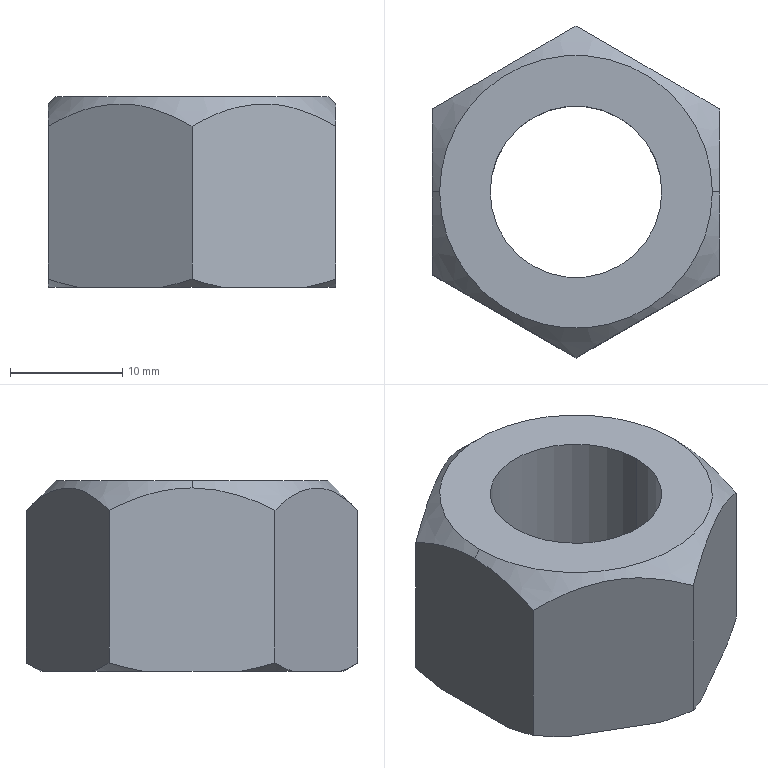Part | SolidWorks | features Cut 2, Chamfer 1, Extrusion 1 | 1 solid | 20 faces | box 25.6 x 29.56 x 17 mm | volume 6436 mm3 | cone 10 | plane 8 | cylinder 2 | commonest cylinder face diameters 15.294 x2
STEP:
#1=CARTESIAN_POINT('',(-12.15,0.,17.));
#2=VERTEX_POINT('',#1);
#3=CARTESIAN_POINT('',(12.15,0.,17.));
#4=VERTEX_POINT('',#3);
#5=CARTESIAN_POINT('',(0.,0.,17.));
#6=DIRECTION('',(0.,0.,1.));
#7=DIRECTION('',(1.,0.,0.));
#8=AXIS2_PLACEMENT_3D('',#5,#6,#7);
#9=CIRCLE('',#8,12.15);
#10=EDGE_CURVE('',#2,#4,#9,.T.);
#11=ORIENTED_EDGE('',*,*,#10,.F.);
#12=CARTESIAN_POINT('',(-12.8,0.,16.35));
#13=VERTEX_POINT('',#12);
#14=CARTESIAN_POINT('',(-12.15,0.,17.));
#15=DIRECTION('',(-0.7071,0.,-0.7071));
#16=VECTOR('',#15,1000.);
#17=LINE('',#14,#16);
#18=EDGE_CURVE('',#2,#13,#17,.T.);
#19=ORIENTED_EDGE('',*,*,#18,.T.);
#20=CARTESIAN_POINT('',(-12.8,-7.39,14.37));
#21=VERTEX_POINT('',#20);
#22=CARTESIAN_POINT('',(-12.8,0.,16.35));
#23=CARTESIAN_POINT('',(-12.8,-0.3244,16.35));
#24=CARTESIAN_POINT('',(-12.8,-0.6506,16.338));
#25=CARTESIAN_POINT('',(-12.8,-1.295,16.289));
#26=CARTESIAN_POINT('',(-12.8,-1.614,16.253));
#27=CARTESIAN_POINT('',(-12.8,-2.565,16.111));
#28=CARTESIAN_POINT('',(-12.8,-3.189,15.972));
#29=CARTESIAN_POINT('',(-12.8,-4.421,15.621));
#30=CARTESIAN_POINT('',(-12.8,-5.03,15.408));
#31=CARTESIAN_POINT('',(-12.8,-6.232,14.924));
#32=CARTESIAN_POINT('',(-12.8,-6.817,14.657));
#33=CARTESIAN_POINT('',(-12.8,-7.39,14.37));
#34=B_SPLINE_CURVE_WITH_KNOTS('',3,(#22,#23,#24,#25,#26,#27,#28,#29,#30,#31,#32,#33),.UNSPECIFIED.,.F.,.F.,(4,2,2,2,2,4),(0.01548,0.01644,0.0174,0.01931,0.02122,0.02314),.UNSPECIFIED.);
#35=EDGE_CURVE('',#13,#21,#34,.T.);
#36=ORIENTED_EDGE('',*,*,#35,.T.);
#37=CARTESIAN_POINT('',(0.,-14.78,14.37));
#38=VERTEX_POINT('',#37);
#39=CARTESIAN_POINT('',(-12.8,-7.39,14.37));
#40=CARTESIAN_POINT('',(-11.8,-7.967,14.947));
#41=CARTESIAN_POINT('',(-10.777,-8.558,15.438));
#42=CARTESIAN_POINT('',(-9.188,-9.475,15.964));
#43=CARTESIAN_POINT('',(-8.649,-9.786,16.104));
#44=CARTESIAN_POINT('',(-7.549,-10.422,16.297));
#45=CARTESIAN_POINT('',(-6.982,-10.749,16.349));
#46=CARTESIAN_POINT('',(-5.306,-11.717,16.353));
#47=CARTESIAN_POINT('',(-4.208,-12.351,16.157));
#48=CARTESIAN_POINT('',(-2.042,-13.601,15.449));
#49=CARTESIAN_POINT('',(-1.006,-14.199,14.951));
#50=CARTESIAN_POINT('',(0.,-14.78,14.37));
#51=B_SPLINE_CURVE_WITH_KNOTS('',3,(#39,#40,#41,#42,#43,#44,#45,#46,#47,#48,#49,#50),.UNSPECIFIED.,.F.,.F.,(4,2,2,2,2,4),(0.000000254,0.003817,0.005725,0.007634,0.01145,0.01527),.UNSPECIFIED.);
#52=EDGE_CURVE('',#21,#38,#51,.T.);
#53=ORIENTED_EDGE('',*,*,#52,.T.);
#54=CARTESIAN_POINT('',(12.8,-7.39,14.37));
#55=VERTEX_POINT('',#54);
#56=CARTESIAN_POINT('',(0.,-14.78,14.37));
#57=CARTESIAN_POINT('',(1.,-14.203,14.947));
#58=CARTESIAN_POINT('',(2.023,-13.612,15.438));
#59=CARTESIAN_POINT('',(3.612,-12.695,15.964));
#60=CARTESIAN_POINT('',(4.15,-12.384,16.104));
#61=CARTESIAN_POINT('',(5.251,-11.748,16.297));
#62=CARTESIAN_POINT('',(5.818,-11.421,16.349));
#63=CARTESIAN_POINT('',(7.494,-10.453,16.353));
#64=CARTESIAN_POINT('',(8.592,-9.819,16.157));
#65=CARTESIAN_POINT('',(10.758,-8.569,15.449));
#66=CARTESIAN_POINT('',(11.794,-7.971,14.951));
#67=CARTESIAN_POINT('',(12.8,-7.39,14.37));
#68=B_SPLINE_CURVE_WITH_KNOTS('',3,(#56,#57,#58,#59,#60,#61,#62,#63,#64,#65,#66,#67),.UNSPECIFIED.,.F.,.F.,(4,2,2,2,2,4),(0.000000254,0.003817,0.005725,0.007634,0.01145,0.01527),.UNSPECIFIED.);
#69=EDGE_CURVE('',#38,#55,#68,.T.);
#70=ORIENTED_EDGE('',*,*,#69,.T.);
#71=CARTESIAN_POINT('',(12.8,0.,16.35));
#72=VERTEX_POINT('',#71);
#73=CARTESIAN_POINT('',(12.8,-7.39,14.37));
#74=CARTESIAN_POINT('',(12.8,-6.817,14.657));
#75=CARTESIAN_POINT('',(12.8,-6.232,14.924));
#76=CARTESIAN_POINT('',(12.8,-5.03,15.408));
#77=CARTESIAN_POINT('',(12.8,-4.421,15.621));
#78=CARTESIAN_POINT('',(12.8,-3.189,15.972));
#79=CARTESIAN_POINT('',(12.8,-2.565,16.111));
#80=CARTESIAN_POINT('',(12.8,-1.614,16.253));
#81=CARTESIAN_POINT('',(12.8,-1.295,16.289));
#82=CARTESIAN_POINT('',(12.8,-0.6506,16.338));
#83=CARTESIAN_POINT('',(12.8,-0.3244,16.35));
#84=CARTESIAN_POINT('',(12.8,0.,16.35));
#85=B_SPLINE_CURVE_WITH_KNOTS('',3,(#73,#74,#75,#76,#77,#78,#79,#80,#81,#82,#83,#84),.UNSPECIFIED.,.F.,.F.,(4,2,2,2,2,4),(0.009846,0.01176,0.01368,0.01559,0.01655,0.0175),.UNSPECIFIED.);
#86=EDGE_CURVE('',#55,#72,#85,.T.);
#87=ORIENTED_EDGE('',*,*,#86,.T.);
#88=CARTESIAN_POINT('',(12.15,0.,17.));
#89=DIRECTION('',(0.7071,0.,-0.7071));
#90=VECTOR('',#89,1000.);
#91=LINE('',#88,#90);
#92=EDGE_CURVE('',#4,#72,#91,.T.);
#93=ORIENTED_EDGE('',*,*,#92,.F.);
#94=EDGE_LOOP('',(#11,#19,#36,#53,#70,#87,#93));
#95=FACE_OUTER_BOUND('',#94,.T.);
#96=CARTESIAN_POINT('',(0.,0.,17.));
#97=DIRECTION('',(0.,0.,-1.));
#98=DIRECTION('',(1.,0.,0.));
#99=AXIS2_PLACEMENT_3D('',#96,#97,#98);
#100=CONICAL_SURFACE('',#99,12.15,0.7854);
#101=ADVANCED_FACE('',(#95),#100,.T.);
#102=CARTESIAN_POINT('',(7.647,0.,0.2946));
#103=VERTEX_POINT('',#102);
#104=CARTESIAN_POINT('',(-7.647,0.,0.2946));
#105=VERTEX_POINT('',#104);
#106=CARTESIAN_POINT('',(0.,0.,0.2946));
#107=DIRECTION('',(0.,0.,-1.));
#108=DIRECTION('',(-1.,0.,0.));
#109=AXIS2_PLACEMENT_3D('',#106,#107,#108);
#110=CIRCLE('',#109,7.647);
#111=EDGE_CURVE('',#103,#105,#110,.T.);
#112=ORIENTED_EDGE('',*,*,#111,.F.);
#113=CARTESIAN_POINT('',(7.942,0.,0.));
#114=VERTEX_POINT('',#113);
#115=CARTESIAN_POINT('',(7.942,0.,0.));
#116=DIRECTION('',(0.7071,0.,-0.7071));
#117=VECTOR('',#116,1000.);
#118=LINE('',#115,#117);
#119=EDGE_CURVE('',#103,#114,#118,.T.);
#120=ORIENTED_EDGE('',*,*,#119,.T.);
#121=CARTESIAN_POINT('',(-7.942,0.,0.));
#122=VERTEX_POINT('',#121);
#123=CARTESIAN_POINT('',(0.,0.,0.));
#124=DIRECTION('',(0.,0.,1.));
#125=DIRECTION('',(-1.,0.,0.));
#126=AXIS2_PLACEMENT_3D('',#123,#124,#125);
#127=CIRCLE('',#126,7.942);
#128=EDGE_CURVE('',#122,#114,#127,.T.);
#129=ORIENTED_EDGE('',*,*,#128,.F.);
#130=CARTESIAN_POINT('',(-7.942,0.,0.));
#131=DIRECTION('',(-0.7071,0.,-0.7071));
#132=VECTOR('',#131,1000.);
#133=LINE('',#130,#132);
#134=EDGE_CURVE('',#105,#122,#133,.T.);
#135=ORIENTED_EDGE('',*,*,#134,.F.);
#136=EDGE_LOOP('',(#112,#120,#129,#135));
#137=FACE_OUTER_BOUND('',#136,.T.);
#138=CARTESIAN_POINT('',(0.,0.,0.));
#139=DIRECTION('',(0.,0.,-1.));
#140=DIRECTION('',(-1.,0.,0.));
#141=AXIS2_PLACEMENT_3D('',#138,#139,#140);
#142=CONICAL_SURFACE('',#141,7.942,0.7854);
#143=ADVANCED_FACE('',(#137),#142,.F.);
#144=CARTESIAN_POINT('',(-7.647,0.,17.));
#145=VERTEX_POINT('',#144);
#146=CARTESIAN_POINT('',(7.647,0.,17.));
#147=VERTEX_POINT('',#146);
#148=CARTESIAN_POINT('',(0.,0.,17.));
#149=DIRECTION('',(0.,0.,1.));
#150=DIRECTION('',(1.,0.,0.));
#151=AXIS2_PLACEMENT_3D('',#148,#149,#150);
#152=CIRCLE('',#151,7.647);
#153=EDGE_CURVE('',#145,#147,#152,.T.);
#154=ORIENTED_EDGE('',*,*,#153,.T.);
#155=CARTESIAN_POINT('',(7.647,0.,17.));
#156=DIRECTION('',(0.,0.,-1.));
#157=VECTOR('',#156,1000.);
#158=LINE('',#155,#157);
#159=EDGE_CURVE('',#147,#103,#158,.T.);
#160=ORIENTED_EDGE('',*,*,#159,.T.);
#161=ORIENTED_EDGE('',*,*,#111,.T.);
#162=CARTESIAN_POINT('',(-7.647,0.,17.));
#163=DIRECTION('',(0.,0.,-1.));
#164=VECTOR('',#163,1000.);
#165=LINE('',#162,#164);
#166=EDGE_CURVE('',#145,#105,#165,.T.);
#167=ORIENTED_EDGE('',*,*,#166,.F.);
#168=EDGE_LOOP('',(#154,#160,#161,#167));
#169=FACE_OUTER_BOUND('',#168,.T.);
#170=CARTESIAN_POINT('',(0.,0.,17.));
#171=DIRECTION('',(0.,0.,-1.));
#172=DIRECTION('',(-1.,0.,0.));
#173=AXIS2_PLACEMENT_3D('',#170,#171,#172);
#174=CYLINDRICAL_SURFACE('',#173,7.647);
#175=ADVANCED_FACE('',(#169),#174,.F.);
#176=CARTESIAN_POINT('',(12.8,7.39,14.37));
#177=VERTEX_POINT('',#176);
#178=CARTESIAN_POINT('',(0.,14.78,14.37));
#179=VERTEX_POINT('',#178);
#180=CARTESIAN_POINT('',(12.8,7.39,14.37));
#181=CARTESIAN_POINT('',(11.8,7.967,14.947));
#182=CARTESIAN_POINT('',(10.777,8.558,15.438));
#183=CARTESIAN_POINT('',(9.188,9.475,15.964));
#184=CARTESIAN_POINT('',(8.649,9.786,16.104));
#185=CARTESIAN_POINT('',(7.549,10.422,16.297));
#186=CARTESIAN_POINT('',(6.982,10.749,16.349));
#187=CARTESIAN_POINT('',(5.306,11.717,16.353));
#188=CARTESIAN_POINT('',(4.208,12.351,16.157));
#189=CARTESIAN_POINT('',(2.042,13.601,15.449));
#190=CARTESIAN_POINT('',(1.006,14.199,14.951));
#191=CARTESIAN_POINT('',(0.,14.78,14.37));
#192=B_SPLINE_CURVE_WITH_KNOTS('',3,(#180,#181,#182,#183,#184,#185,#186,#187,#188,#189,#190,#191),.UNSPECIFIED.,.F.,.F.,(4,2,2,2,2,4),(0.000000254,0.003817,0.005725,0.007634,0.01145,0.01527),.UNSPECIFIED.);
#193=EDGE_CURVE('',#177,#179,#192,.T.);
#194=ORIENTED_EDGE('',*,*,#193,.F.);
#195=CARTESIAN_POINT('',(12.8,7.39,0.739));
#196=VERTEX_POINT('',#195);
#197=CARTESIAN_POINT('',(12.8,7.39,17.));
#198=DIRECTION('',(0.,0.,-1.));
#199=VECTOR('',#198,1000.);
#200=LINE('',#197,#199);
#201=EDGE_CURVE('',#177,#196,#200,.T.);
#202=ORIENTED_EDGE('',*,*,#201,.T.);
#203=CARTESIAN_POINT('',(10.116,8.939,0.));
#204=VERTEX_POINT('',#203);
#205=CARTESIAN_POINT('',(10.116,8.939,0.));
#206=CARTESIAN_POINT('',(11.02,8.418,0.1915));
#207=CARTESIAN_POINT('',(11.913,7.902,0.4435));
#208=CARTESIAN_POINT('',(12.8,7.39,0.739));
#209=B_SPLINE_CURVE_WITH_KNOTS('',3,(#205,#206,#207,#208),.UNSPECIFIED.,.F.,.F.,(4,4),(0.02758,0.03077),.UNSPECIFIED.);
#210=EDGE_CURVE('',#204,#196,#209,.T.);
#211=ORIENTED_EDGE('',*,*,#210,.F.);
#212=CARTESIAN_POINT('',(2.684,13.231,0.));
#213=VERTEX_POINT('',#212);
#214=CARTESIAN_POINT('',(12.8,7.39,0.));
#215=DIRECTION('',(-0.866,0.5,0.));
#216=VECTOR('',#215,1000.);
#217=LINE('',#214,#216);
#218=EDGE_CURVE('',#204,#213,#217,.T.);
#219=ORIENTED_EDGE('',*,*,#218,.T.);
#220=CARTESIAN_POINT('',(0.,14.78,0.739));
#221=VERTEX_POINT('',#220);
#222=CARTESIAN_POINT('',(0.,14.78,0.739));
#223=CARTESIAN_POINT('',(0.8872,14.268,0.4433));
#224=CARTESIAN_POINT('',(1.781,13.752,0.1913));
#225=CARTESIAN_POINT('',(2.684,13.231,0.));
#226=B_SPLINE_CURVE_WITH_KNOTS('',3,(#222,#223,#224,#225),.UNSPECIFIED.,.F.,.F.,(4,4),(0.01574,0.01894),.UNSPECIFIED.);
#227=EDGE_CURVE('',#221,#213,#226,.T.);
#228=ORIENTED_EDGE('',*,*,#227,.F.);
#229=CARTESIAN_POINT('',(0.,14.78,17.));
#230=DIRECTION('',(0.,0.,-1.));
#231=VECTOR('',#230,1000.);
#232=LINE('',#229,#231);
#233=EDGE_CURVE('',#179,#221,#232,.T.);
#234=ORIENTED_EDGE('',*,*,#233,.F.);
#235=EDGE_LOOP('',(#194,#202,#211,#219,#228,#234));
#236=FACE_OUTER_BOUND('',#235,.T.);
#237=CARTESIAN_POINT('',(12.8,7.39,17.));
#238=DIRECTION('',(-0.5,-0.866,0.));
#239=DIRECTION('',(0.866,-0.5,0.));
#240=AXIS2_PLACEMENT_3D('',#237,#238,#239);
#241=PLANE('',#240);
#242=ADVANCED_FACE('',(#236),#241,.F.);
#243=CARTESIAN_POINT('',(-12.8,7.39,14.37));
#244=VERTEX_POINT('',#243);
#245=CARTESIAN_POINT('',(0.,14.78,14.37));
#246=CARTESIAN_POINT('',(-1.,14.203,14.947));
#247=CARTESIAN_POINT('',(-2.023,13.612,15.438));
#248=CARTESIAN_POINT('',(-3.612,12.695,15.964));
#249=CARTESIAN_POINT('',(-4.15,12.384,16.104));
#250=CARTESIAN_POINT('',(-5.251,11.748,16.297));
#251=CARTESIAN_POINT('',(-5.818,11.421,16.349));
#252=CARTESIAN_POINT('',(-7.494,10.453,16.353));
#253=CARTESIAN_POINT('',(-8.592,9.819,16.157));
#254=CARTESIAN_POINT('',(-10.758,8.569,15.449));
#255=CARTESIAN_POINT('',(-11.794,7.971,14.951));
#256=CARTESIAN_POINT('',(-12.8,7.39,14.37));
#257=B_SPLINE_CURVE_WITH_KNOTS('',3,(#245,#246,#247,#248,#249,#250,#251,#252,#253,#254,#255,#256),.UNSPECIFIED.,.F.,.F.,(4,2,2,2,2,4),(0.000000254,0.003817,0.005725,0.007634,0.01145,0.01527),.UNSPECIFIED.);
#258=EDGE_CURVE('',#179,#244,#257,.T.);
#259=ORIENTED_EDGE('',*,*,#258,.F.);
#260=ORIENTED_EDGE('',*,*,#233,.T.);
#261=CARTESIAN_POINT('',(-2.684,13.231,0.));
#262=VERTEX_POINT('',#261);
#263=CARTESIAN_POINT('',(-2.684,13.231,0.));
#264=CARTESIAN_POINT('',(-1.78,13.752,0.1915));
#265=CARTESIAN_POINT('',(-0.8864,14.268,0.4435));
#266=CARTESIAN_POINT('',(0.,14.78,0.739));
#267=B_SPLINE_CURVE_WITH_KNOTS('',3,(#263,#264,#265,#266),.UNSPECIFIED.,.F.,.F.,(4,4),(0.02758,0.03077),.UNSPECIFIED.);
#268=EDGE_CURVE('',#262,#221,#267,.T.);
#269=ORIENTED_EDGE('',*,*,#268,.F.);
#270=CARTESIAN_POINT('',(-10.116,8.939,0.));
#271=VERTEX_POINT('',#270);
#272=CARTESIAN_POINT('',(0.,14.78,0.));
#273=DIRECTION('',(-0.866,-0.5,0.));
#274=VECTOR('',#273,1000.);
#275=LINE('',#272,#274);
#276=EDGE_CURVE('',#262,#271,#275,.T.);
#277=ORIENTED_EDGE('',*,*,#276,.T.);
#278=CARTESIAN_POINT('',(-12.8,7.39,0.739));
#279=VERTEX_POINT('',#278);
#280=CARTESIAN_POINT('',(-12.8,7.39,0.739));
#281=CARTESIAN_POINT('',(-11.913,7.902,0.4433));
#282=CARTESIAN_POINT('',(-11.019,8.418,0.1913));
#283=CARTESIAN_POINT('',(-10.116,8.939,0.));
#284=B_SPLINE_CURVE_WITH_KNOTS('',3,(#280,#281,#282,#283),.UNSPECIFIED.,.F.,.F.,(4,4),(0.01574,0.01894),.UNSPECIFIED.);
#285=EDGE_CURVE('',#279,#271,#284,.T.);
#286=ORIENTED_EDGE('',*,*,#285,.F.);
#287=CARTESIAN_POINT('',(-12.8,7.39,17.));
#288=DIRECTION('',(0.,0.,-1.));
#289=VECTOR('',#288,1000.);
#290=LINE('',#287,#289);
#291=EDGE_CURVE('',#244,#279,#290,.T.);
#292=ORIENTED_EDGE('',*,*,#291,.F.);
#293=EDGE_LOOP('',(#259,#260,#269,#277,#286,#292));
#294=FACE_OUTER_BOUND('',#293,.T.);
#295=CARTESIAN_POINT('',(0.,14.78,17.));
#296=DIRECTION('',(0.5,-0.866,0.));
#297=DIRECTION('',(0.866,0.5,0.));
#298=AXIS2_PLACEMENT_3D('',#295,#296,#297);
#299=PLANE('',#298);
#300=ADVANCED_FACE('',(#294),#299,.F.);
#301=CARTESIAN_POINT('',(-12.8,7.39,14.37));
#302=CARTESIAN_POINT('',(-12.8,6.818,14.656));
#303=CARTESIAN_POINT('',(-12.8,6.235,14.923));
#304=CARTESIAN_POINT('',(-12.8,5.039,15.405));
#305=CARTESIAN_POINT('',(-12.8,4.423,15.62));
#306=CARTESIAN_POINT('',(-12.8,2.564,16.15));
#307=CARTESIAN_POINT('',(-12.8,1.299,16.35));
#308=CARTESIAN_POINT('',(-12.8,0.,16.35));
#309=B_SPLINE_CURVE_WITH_KNOTS('',3,(#301,#302,#303,#304,#305,#306,#307,#308),.UNSPECIFIED.,.F.,.F.,(4,2,2,4),(0.007822,0.009738,0.01165,0.01548),.UNSPECIFIED.);
#310=EDGE_CURVE('',#244,#13,#309,.T.);
#311=ORIENTED_EDGE('',*,*,#310,.F.);
#312=ORIENTED_EDGE('',*,*,#291,.T.);
#313=CARTESIAN_POINT('',(-12.8,4.291,0.));
#314=VERTEX_POINT('',#313);
#315=CARTESIAN_POINT('',(-12.8,4.291,0.));
#316=CARTESIAN_POINT('',(-12.8,5.336,0.1918));
#317=CARTESIAN_POINT('',(-12.8,6.368,0.4439));
#318=CARTESIAN_POINT('',(-12.8,7.39,0.739));
#319=B_SPLINE_CURVE_WITH_KNOTS('',3,(#315,#316,#317,#318),.UNSPECIFIED.,.F.,.F.,(4,4),(0.0254,0.02859),.UNSPECIFIED.);
#320=EDGE_CURVE('',#314,#279,#319,.T.);
#321=ORIENTED_EDGE('',*,*,#320,.F.);
#322=CARTESIAN_POINT('',(-12.8,-4.291,0.));
#323=VERTEX_POINT('',#322);
#324=CARTESIAN_POINT('',(-12.8,7.39,0.));
#325=DIRECTION('',(0.,-1.,0.));
#326=VECTOR('',#325,1000.);
#327=LINE('',#324,#326);
#328=EDGE_CURVE('',#314,#323,#327,.T.);
#329=ORIENTED_EDGE('',*,*,#328,.T.);
#330=CARTESIAN_POINT('',(-12.8,-7.39,0.739));
#331=VERTEX_POINT('',#330);
#332=CARTESIAN_POINT('',(-12.8,-7.39,0.739));
#333=CARTESIAN_POINT('',(-12.8,-6.364,0.4427));
#334=CARTESIAN_POINT('',(-12.8,-5.331,0.1909));
#335=CARTESIAN_POINT('',(-12.8,-4.291,0.));
#336=B_SPLINE_CURVE_WITH_KNOTS('',3,(#332,#333,#334,#335),.UNSPECIFIED.,.F.,.F.,(4,4),(0.01358,0.01677),.UNSPECIFIED.);
#337=EDGE_CURVE('',#331,#323,#336,.T.);
#338=ORIENTED_EDGE('',*,*,#337,.F.);
#339=CARTESIAN_POINT('',(-12.8,-7.39,17.));
#340=DIRECTION('',(0.,0.,-1.));
#341=VECTOR('',#340,1000.);
#342=LINE('',#339,#341);
#343=EDGE_CURVE('',#21,#331,#342,.T.);
#344=ORIENTED_EDGE('',*,*,#343,.F.);
#345=ORIENTED_EDGE('',*,*,#35,.F.);
#346=EDGE_LOOP('',(#311,#312,#321,#329,#338,#344,#345));
#347=FACE_OUTER_BOUND('',#346,.T.);
#348=CARTESIAN_POINT('',(-12.8,7.39,17.));
#349=DIRECTION('',(1.,0.,0.));
#350=DIRECTION('',(0.,1.,0.));
#351=AXIS2_PLACEMENT_3D('',#348,#349,#350);
#352=PLANE('',#351);
#353=ADVANCED_FACE('',(#347),#352,.F.);
#354=ORIENTED_EDGE('',*,*,#52,.F.);
#355=ORIENTED_EDGE('',*,*,#343,.T.);
#356=CARTESIAN_POINT('',(-10.116,-8.939,0.));
#357=VERTEX_POINT('',#356);
#358=CARTESIAN_POINT('',(-10.116,-8.939,0.));
#359=CARTESIAN_POINT('',(-11.02,-8.418,0.1915));
#360=CARTESIAN_POINT('',(-11.913,-7.902,0.4435));
#361=CARTESIAN_POINT('',(-12.8,-7.39,0.739));
#362=B_SPLINE_CURVE_WITH_KNOTS('',3,(#358,#359,#360,#361),.UNSPECIFIED.,.F.,.F.,(4,4),(0.02758,0.03077),.UNSPECIFIED.);
#363=EDGE_CURVE('',#357,#331,#362,.T.);
#364=ORIENTED_EDGE('',*,*,#363,.F.);
#365=CARTESIAN_POINT('',(-2.684,-13.231,0.));
#366=VERTEX_POINT('',#365);
#367=CARTESIAN_POINT('',(-12.8,-7.39,0.));
#368=DIRECTION('',(0.866,-0.5,0.));
#369=VECTOR('',#368,1000.);
#370=LINE('',#367,#369);
#371=EDGE_CURVE('',#357,#366,#370,.T.);
#372=ORIENTED_EDGE('',*,*,#371,.T.);
#373=CARTESIAN_POINT('',(0.,-14.78,0.739));
#374=VERTEX_POINT('',#373);
#375=CARTESIAN_POINT('',(0.,-14.78,0.739));
#376=CARTESIAN_POINT('',(-0.8872,-14.268,0.4433));
#377=CARTESIAN_POINT('',(-1.781,-13.752,0.1913));
#378=CARTESIAN_POINT('',(-2.684,-13.231,0.));
#379=B_SPLINE_CURVE_WITH_KNOTS('',3,(#375,#376,#377,#378),.UNSPECIFIED.,.F.,.F.,(4,4),(0.01574,0.01894),.UNSPECIFIED.);
#380=EDGE_CURVE('',#374,#366,#379,.T.);
#381=ORIENTED_EDGE('',*,*,#380,.F.);
#382=CARTESIAN_POINT('',(0.,-14.78,17.));
#383=DIRECTION('',(0.,0.,-1.));
#384=VECTOR('',#383,1000.);
#385=LINE('',#382,#384);
#386=EDGE_CURVE('',#38,#374,#385,.T.);
#387=ORIENTED_EDGE('',*,*,#386,.F.);
#388=EDGE_LOOP('',(#354,#355,#364,#372,#381,#387));
#389=FACE_OUTER_BOUND('',#388,.T.);
#390=CARTESIAN_POINT('',(-12.8,-7.39,17.));
#391=DIRECTION('',(0.5,0.866,0.));
#392=DIRECTION('',(-0.866,0.5,0.));
#393=AXIS2_PLACEMENT_3D('',#390,#391,#392);
#394=PLANE('',#393);
#395=ADVANCED_FACE('',(#389),#394,.F.);
#396=ORIENTED_EDGE('',*,*,#69,.F.);
#397=ORIENTED_EDGE('',*,*,#386,.T.);
#398=CARTESIAN_POINT('',(2.684,-13.231,0.));
#399=VERTEX_POINT('',#398);
#400=CARTESIAN_POINT('',(2.684,-13.231,0.));
#401=CARTESIAN_POINT('',(1.78,-13.752,0.1915));
#402=CARTESIAN_POINT('',(0.8864,-14.268,0.4435));
#403=CARTESIAN_POINT('',(0.,-14.78,0.739));
#404=B_SPLINE_CURVE_WITH_KNOTS('',3,(#400,#401,#402,#403),.UNSPECIFIED.,.F.,.F.,(4,4),(0.02758,0.03077),.UNSPECIFIED.);
#405=EDGE_CURVE('',#399,#374,#404,.T.);
#406=ORIENTED_EDGE('',*,*,#405,.F.);
#407=CARTESIAN_POINT('',(10.116,-8.939,0.));
#408=VERTEX_POINT('',#407);
#409=CARTESIAN_POINT('',(0.,-14.78,0.));
#410=DIRECTION('',(0.866,0.5,0.));
#411=VECTOR('',#410,1000.);
#412=LINE('',#409,#411);
#413=EDGE_CURVE('',#399,#408,#412,.T.);
#414=ORIENTED_EDGE('',*,*,#413,.T.);
#415=CARTESIAN_POINT('',(12.8,-7.39,0.739));
#416=VERTEX_POINT('',#415);
#417=CARTESIAN_POINT('',(12.8,-7.39,0.739));
#418=CARTESIAN_POINT('',(11.913,-7.902,0.4433));
#419=CARTESIAN_POINT('',(11.019,-8.418,0.1913));
#420=CARTESIAN_POINT('',(10.116,-8.939,0.));
#421=B_SPLINE_CURVE_WITH_KNOTS('',3,(#417,#418,#419,#420),.UNSPECIFIED.,.F.,.F.,(4,4),(0.01574,0.01894),.UNSPECIFIED.);
#422=EDGE_CURVE('',#416,#408,#421,.T.);
#423=ORIENTED_EDGE('',*,*,#422,.F.);
#424=CARTESIAN_POINT('',(12.8,-7.39,17.));
#425=DIRECTION('',(0.,0.,-1.));
#426=VECTOR('',#425,1000.);
#427=LINE('',#424,#426);
#428=EDGE_CURVE('',#55,#416,#427,.T.);
#429=ORIENTED_EDGE('',*,*,#428,.F.);
#430=EDGE_LOOP('',(#396,#397,#406,#414,#423,#429));
#431=FACE_OUTER_BOUND('',#430,.T.);
#432=CARTESIAN_POINT('',(0.,-14.78,17.));
#433=DIRECTION('',(-0.5,0.866,0.));
#434=DIRECTION('',(-0.866,-0.5,0.));
#435=AXIS2_PLACEMENT_3D('',#432,#433,#434);
#436=PLANE('',#435);
#437=ADVANCED_FACE('',(#431),#436,.F.);
#438=ORIENTED_EDGE('',*,*,#86,.F.);
#439=ORIENTED_EDGE('',*,*,#428,.T.);
#440=CARTESIAN_POINT('',(12.8,-4.291,0.));
#441=VERTEX_POINT('',#440);
#442=CARTESIAN_POINT('',(12.8,-4.291,0.));
#443=CARTESIAN_POINT('',(12.8,-5.336,0.1918));
#444=CARTESIAN_POINT('',(12.8,-6.368,0.4439));
#445=CARTESIAN_POINT('',(12.8,-7.39,0.739));
#446=B_SPLINE_CURVE_WITH_KNOTS('',3,(#442,#443,#444,#445),.UNSPECIFIED.,.F.,.F.,(4,4),(0.0254,0.02859),.UNSPECIFIED.);
#447=EDGE_CURVE('',#441,#416,#446,.T.);
#448=ORIENTED_EDGE('',*,*,#447,.F.);
#449=CARTESIAN_POINT('',(12.8,4.291,0.));
#450=VERTEX_POINT('',#449);
#451=CARTESIAN_POINT('',(12.8,-7.39,0.));
#452=DIRECTION('',(0.,1.,0.));
#453=VECTOR('',#452,1000.);
#454=LINE('',#451,#453);
#455=EDGE_CURVE('',#441,#450,#454,.T.);
#456=ORIENTED_EDGE('',*,*,#455,.T.);
#457=CARTESIAN_POINT('',(12.8,7.39,0.739));
#458=CARTESIAN_POINT('',(12.8,6.364,0.4427));
#459=CARTESIAN_POINT('',(12.8,5.331,0.1909));
#460=CARTESIAN_POINT('',(12.8,4.291,0.));
#461=B_SPLINE_CURVE_WITH_KNOTS('',3,(#457,#458,#459,#460),.UNSPECIFIED.,.F.,.F.,(4,4),(0.01358,0.01677),.UNSPECIFIED.);
#462=EDGE_CURVE('',#196,#450,#461,.T.);
#463=ORIENTED_EDGE('',*,*,#462,.F.);
#464=ORIENTED_EDGE('',*,*,#201,.F.);
#465=CARTESIAN_POINT('',(12.8,0.,16.35));
#466=CARTESIAN_POINT('',(12.8,1.299,16.35));
#467=CARTESIAN_POINT('',(12.8,2.564,16.15));
#468=CARTESIAN_POINT('',(12.8,4.423,15.62));
#469=CARTESIAN_POINT('',(12.8,5.039,15.405));
#470=CARTESIAN_POINT('',(12.8,6.235,14.923));
#471=CARTESIAN_POINT('',(12.8,6.818,14.656));
#472=CARTESIAN_POINT('',(12.8,7.39,14.37));
#473=B_SPLINE_CURVE_WITH_KNOTS('',3,(#465,#466,#467,#468,#469,#470,#471,#472),.UNSPECIFIED.,.F.,.F.,(4,2,2,4),(0.0175,0.02134,0.02325,0.02517),.UNSPECIFIED.);
#474=EDGE_CURVE('',#72,#177,#473,.T.);
#475=ORIENTED_EDGE('',*,*,#474,.F.);
#476=EDGE_LOOP('',(#438,#439,#448,#456,#463,#464,#475));
#477=FACE_OUTER_BOUND('',#476,.T.);
#478=CARTESIAN_POINT('',(12.8,-7.39,17.));
#479=DIRECTION('',(-1.,0.,0.));
#480=DIRECTION('',(0.,-1.,0.));
#481=AXIS2_PLACEMENT_3D('',#478,#479,#480);
#482=PLANE('',#481);
#483=ADVANCED_FACE('',(#477),#482,.F.);
#484=ORIENTED_EDGE('',*,*,#153,.F.);
#485=CARTESIAN_POINT('',(0.,0.,17.));
#486=DIRECTION('',(0.,0.,1.));
#487=DIRECTION('',(1.,0.,0.));
#488=AXIS2_PLACEMENT_3D('',#485,#486,#487);
#489=CIRCLE('',#488,7.647);
#490=EDGE_CURVE('',#147,#145,#489,.T.);
#491=ORIENTED_EDGE('',*,*,#490,.F.);
#492=EDGE_LOOP('',(#484,#491));
#493=FACE_BOUND('',#492,.T.);
#494=CARTESIAN_POINT('',(0.,0.,17.));
#495=DIRECTION('',(0.,0.,1.));
#496=DIRECTION('',(1.,0.,0.));
#497=AXIS2_PLACEMENT_3D('',#494,#495,#496);
#498=CIRCLE('',#497,12.15);
#499=EDGE_CURVE('',#4,#2,#498,.T.);
#500=ORIENTED_EDGE('',*,*,#499,.T.);
#501=ORIENTED_EDGE('',*,*,#10,.T.);
#502=EDGE_LOOP('',(#500,#501));
#503=FACE_OUTER_BOUND('',#502,.T.);
#504=CARTESIAN_POINT('',(25.6,0.,17.));
#505=DIRECTION('',(0.,0.,-1.));
#506=DIRECTION('',(-1.,0.,0.));
#507=AXIS2_PLACEMENT_3D('',#504,#505,#506);
#508=PLANE('',#507);
#509=ADVANCED_FACE('',(#493,#503),#508,.F.);
#510=ORIENTED_EDGE('',*,*,#128,.T.);
#511=CARTESIAN_POINT('',(0.,0.,0.));
#512=DIRECTION('',(0.,0.,1.));
#513=DIRECTION('',(-1.,0.,0.));
#514=AXIS2_PLACEMENT_3D('',#511,#512,#513);
#515=CIRCLE('',#514,7.942);
#516=EDGE_CURVE('',#114,#122,#515,.T.);
#517=ORIENTED_EDGE('',*,*,#516,.T.);
#518=EDGE_LOOP('',(#510,#517));
#519=FACE_BOUND('',#518,.T.);
#520=ORIENTED_EDGE('',*,*,#328,.F.);
#521=CARTESIAN_POINT('',(0.,0.,0.));
#522=DIRECTION('',(0.,0.,-1.));
#523=DIRECTION('',(-1.,0.,0.));
#524=AXIS2_PLACEMENT_3D('',#521,#522,#523);
#525=CIRCLE('',#524,13.5);
#526=EDGE_CURVE('',#314,#271,#525,.T.);
#527=ORIENTED_EDGE('',*,*,#526,.T.);
#528=ORIENTED_EDGE('',*,*,#276,.F.);
#529=CARTESIAN_POINT('',(0.,0.,0.));
#530=DIRECTION('',(0.,0.,-1.));
#531=DIRECTION('',(-1.,0.,0.));
#532=AXIS2_PLACEMENT_3D('',#529,#530,#531);
#533=CIRCLE('',#532,13.5);
#534=EDGE_CURVE('',#262,#213,#533,.T.);
#535=ORIENTED_EDGE('',*,*,#534,.T.);
#536=ORIENTED_EDGE('',*,*,#218,.F.);
#537=CARTESIAN_POINT('',(0.,0.,0.));
#538=DIRECTION('',(0.,0.,-1.));
#539=DIRECTION('',(-1.,0.,0.));
#540=AXIS2_PLACEMENT_3D('',#537,#538,#539);
#541=CIRCLE('',#540,13.5);
#542=EDGE_CURVE('',#204,#450,#541,.T.);
#543=ORIENTED_EDGE('',*,*,#542,.T.);
#544=ORIENTED_EDGE('',*,*,#455,.F.);
#545=CARTESIAN_POINT('',(0.,0.,0.));
#546=DIRECTION('',(0.,0.,-1.));
#547=DIRECTION('',(-1.,0.,0.));
#548=AXIS2_PLACEMENT_3D('',#545,#546,#547);
#549=CIRCLE('',#548,13.5);
#550=EDGE_CURVE('',#441,#408,#549,.T.);
#551=ORIENTED_EDGE('',*,*,#550,.T.);
#552=ORIENTED_EDGE('',*,*,#413,.F.);
#553=CARTESIAN_POINT('',(0.,0.,0.));
#554=DIRECTION('',(0.,0.,-1.));
#555=DIRECTION('',(-1.,0.,0.));
#556=AXIS2_PLACEMENT_3D('',#553,#554,#555);
#557=CIRCLE('',#556,13.5);
#558=EDGE_CURVE('',#399,#366,#557,.T.);
#559=ORIENTED_EDGE('',*,*,#558,.T.);
#560=ORIENTED_EDGE('',*,*,#371,.F.);
#561=CARTESIAN_POINT('',(0.,0.,0.));
#562=DIRECTION('',(0.,0.,-1.));
#563=DIRECTION('',(-1.,0.,0.));
#564=AXIS2_PLACEMENT_3D('',#561,#562,#563);
#565=CIRCLE('',#564,13.5);
#566=EDGE_CURVE('',#357,#323,#565,.T.);
#567=ORIENTED_EDGE('',*,*,#566,.T.);
#568=EDGE_LOOP('',(#520,#527,#528,#535,#536,#543,#544,#551,#552,#559,#560,#567));
#569=FACE_OUTER_BOUND('',#568,.T.);
#570=CARTESIAN_POINT('',(25.6,0.,0.));
#571=DIRECTION('',(0.,0.,-1.));
#572=DIRECTION('',(-1.,0.,0.));
#573=AXIS2_PLACEMENT_3D('',#570,#571,#572);
#574=PLANE('',#573);
#575=ADVANCED_FACE('',(#519,#569),#574,.T.);
#576=ORIENTED_EDGE('',*,*,#159,.F.);
#577=ORIENTED_EDGE('',*,*,#490,.T.);
#578=ORIENTED_EDGE('',*,*,#166,.T.);
#579=CARTESIAN_POINT('',(0.,0.,0.2946));
#580=DIRECTION('',(0.,0.,-1.));
#581=DIRECTION('',(-1.,0.,0.));
#582=AXIS2_PLACEMENT_3D('',#579,#580,#581);
#583=CIRCLE('',#582,7.647);
#584=EDGE_CURVE('',#105,#103,#583,.T.);
#585=ORIENTED_EDGE('',*,*,#584,.T.);
#586=EDGE_LOOP('',(#576,#577,#578,#585));
#587=FACE_OUTER_BOUND('',#586,.T.);
#588=CARTESIAN_POINT('',(0.,0.,17.));
#589=DIRECTION('',(0.,0.,-1.));
#590=DIRECTION('',(-1.,0.,0.));
#591=AXIS2_PLACEMENT_3D('',#588,#589,#590);
#592=CYLINDRICAL_SURFACE('',#591,7.647);
#593=ADVANCED_FACE('',(#587),#592,.F.);
#594=ORIENTED_EDGE('',*,*,#422,.T.);
#595=ORIENTED_EDGE('',*,*,#550,.F.);
#596=ORIENTED_EDGE('',*,*,#447,.T.);
#597=EDGE_LOOP('',(#594,#595,#596));
#598=FACE_OUTER_BOUND('',#597,.T.);
#599=CARTESIAN_POINT('',(0.,0.,0.));
#600=DIRECTION('',(0.,0.,1.));
#601=DIRECTION('',(-1.,0.,0.));
#602=AXIS2_PLACEMENT_3D('',#599,#600,#601);
#603=CONICAL_SURFACE('',#602,13.5,1.047);
#604=ADVANCED_FACE('',(#598),#603,.T.);
#605=ORIENTED_EDGE('',*,*,#210,.T.);
#606=ORIENTED_EDGE('',*,*,#462,.T.);
#607=ORIENTED_EDGE('',*,*,#542,.F.);
#608=EDGE_LOOP('',(#605,#606,#607));
#609=FACE_OUTER_BOUND('',#608,.T.);
#610=CARTESIAN_POINT('',(0.,0.,0.));
#611=DIRECTION('',(0.,0.,1.));
#612=DIRECTION('',(-1.,0.,0.));
#613=AXIS2_PLACEMENT_3D('',#610,#611,#612);
#614=CONICAL_SURFACE('',#613,13.5,1.047);
#615=ADVANCED_FACE('',(#609),#614,.T.);
#616=ORIENTED_EDGE('',*,*,#380,.T.);
#617=ORIENTED_EDGE('',*,*,#558,.F.);
#618=ORIENTED_EDGE('',*,*,#405,.T.);
#619=EDGE_LOOP('',(#616,#617,#618));
#620=FACE_OUTER_BOUND('',#619,.T.);
#621=CARTESIAN_POINT('',(0.,0.,0.));
#622=DIRECTION('',(0.,0.,1.));
#623=DIRECTION('',(-1.,0.,0.));
#624=AXIS2_PLACEMENT_3D('',#621,#622,#623);
#625=CONICAL_SURFACE('',#624,13.5,1.047);
#626=ADVANCED_FACE('',(#620),#625,.T.);
#627=ORIENTED_EDGE('',*,*,#337,.T.);
#628=ORIENTED_EDGE('',*,*,#566,.F.);
#629=ORIENTED_EDGE('',*,*,#363,.T.);
#630=EDGE_LOOP('',(#627,#628,#629));
#631=FACE_OUTER_BOUND('',#630,.T.);
#632=CARTESIAN_POINT('',(0.,0.,0.));
#633=DIRECTION('',(0.,0.,1.));
#634=DIRECTION('',(-1.,0.,0.));
#635=AXIS2_PLACEMENT_3D('',#632,#633,#634);
#636=CONICAL_SURFACE('',#635,13.5,1.047);
#637=ADVANCED_FACE('',(#631),#636,.T.);
#638=ORIENTED_EDGE('',*,*,#285,.T.);
#639=ORIENTED_EDGE('',*,*,#526,.F.);
#640=ORIENTED_EDGE('',*,*,#320,.T.);
#641=EDGE_LOOP('',(#638,#639,#640));
#642=FACE_OUTER_BOUND('',#641,.T.);
#643=CARTESIAN_POINT('',(0.,0.,0.));
#644=DIRECTION('',(0.,0.,1.));
#645=DIRECTION('',(-1.,0.,0.));
#646=AXIS2_PLACEMENT_3D('',#643,#644,#645);
#647=CONICAL_SURFACE('',#646,13.5,1.047);
#648=ADVANCED_FACE('',(#642),#647,.T.);
#649=ORIENTED_EDGE('',*,*,#227,.T.);
#650=ORIENTED_EDGE('',*,*,#534,.F.);
#651=ORIENTED_EDGE('',*,*,#268,.T.);
#652=EDGE_LOOP('',(#649,#650,#651));
#653=FACE_OUTER_BOUND('',#652,.T.);
#654=CARTESIAN_POINT('',(0.,0.,0.));
#655=DIRECTION('',(0.,0.,1.));
#656=DIRECTION('',(-1.,0.,0.));
#657=AXIS2_PLACEMENT_3D('',#654,#655,#656);
#658=CONICAL_SURFACE('',#657,13.5,1.047);
#659=ADVANCED_FACE('',(#653),#658,.T.);
#660=ORIENTED_EDGE('',*,*,#119,.F.);
#661=ORIENTED_EDGE('',*,*,#584,.F.);
#662=ORIENTED_EDGE('',*,*,#134,.T.);
#663=ORIENTED_EDGE('',*,*,#516,.F.);
#664=EDGE_LOOP('',(#660,#661,#662,#663));
#665=FACE_OUTER_BOUND('',#664,.T.);
#666=CARTESIAN_POINT('',(0.,0.,0.));
#667=DIRECTION('',(0.,0.,-1.));
#668=DIRECTION('',(-1.,0.,0.));
#669=AXIS2_PLACEMENT_3D('',#666,#667,#668);
#670=CONICAL_SURFACE('',#669,7.942,0.7854);
#671=ADVANCED_FACE('',(#665),#670,.F.);
#672=ORIENTED_EDGE('',*,*,#18,.F.);
#673=ORIENTED_EDGE('',*,*,#499,.F.);
#674=ORIENTED_EDGE('',*,*,#92,.T.);
#675=ORIENTED_EDGE('',*,*,#474,.T.);
#676=ORIENTED_EDGE('',*,*,#193,.T.);
#677=ORIENTED_EDGE('',*,*,#258,.T.);
#678=ORIENTED_EDGE('',*,*,#310,.T.);
#679=EDGE_LOOP('',(#672,#673,#674,#675,#676,#677,#678));
#680=FACE_OUTER_BOUND('',#679,.T.);
#681=CARTESIAN_POINT('',(0.,0.,17.));
#682=DIRECTION('',(0.,0.,-1.));
#683=DIRECTION('',(1.,0.,0.));
#684=AXIS2_PLACEMENT_3D('',#681,#682,#683);
#685=CONICAL_SURFACE('',#684,12.15,0.7854);
#686=ADVANCED_FACE('',(#680),#685,.T.);
#687=CLOSED_SHELL('',(#101,#143,#175,#242,#300,#353,#395,#437,#483,#509,#575,#593,#604,#615,#626,#637,#648,#659,#671,#686));
#688=MANIFOLD_SOLID_BREP('',#687);
#689=CARTESIAN_POINT('',(0.,0.,0.));
#690=DIRECTION('',(0.,0.,1.));
#691=DIRECTION('',(1.,0.,0.));
#692=AXIS2_PLACEMENT_3D('',#689,#690,#691);
#693=(LENGTH_UNIT()NAMED_UNIT(*)SI_UNIT(.MILLI.,.METRE.));
#694=UNCERTAINTY_MEASURE_WITH_UNIT(LENGTH_MEASURE(0.00001),#693,'','');
#695=(NAMED_UNIT(*)PLANE_ANGLE_UNIT()SI_UNIT($,.RADIAN.));
#696=(NAMED_UNIT(*)SI_UNIT($,.STERADIAN.)SOLID_ANGLE_UNIT());
#697=(GEOMETRIC_REPRESENTATION_CONTEXT(3)GLOBAL_UNCERTAINTY_ASSIGNED_CONTEXT((#694))GLOBAL_UNIT_ASSIGNED_CONTEXT((#693,#695,#696))REPRESENTATION_CONTEXT('',''));
#698=ADVANCED_BREP_SHAPE_REPRESENTATION('',(#688,#692),#697);